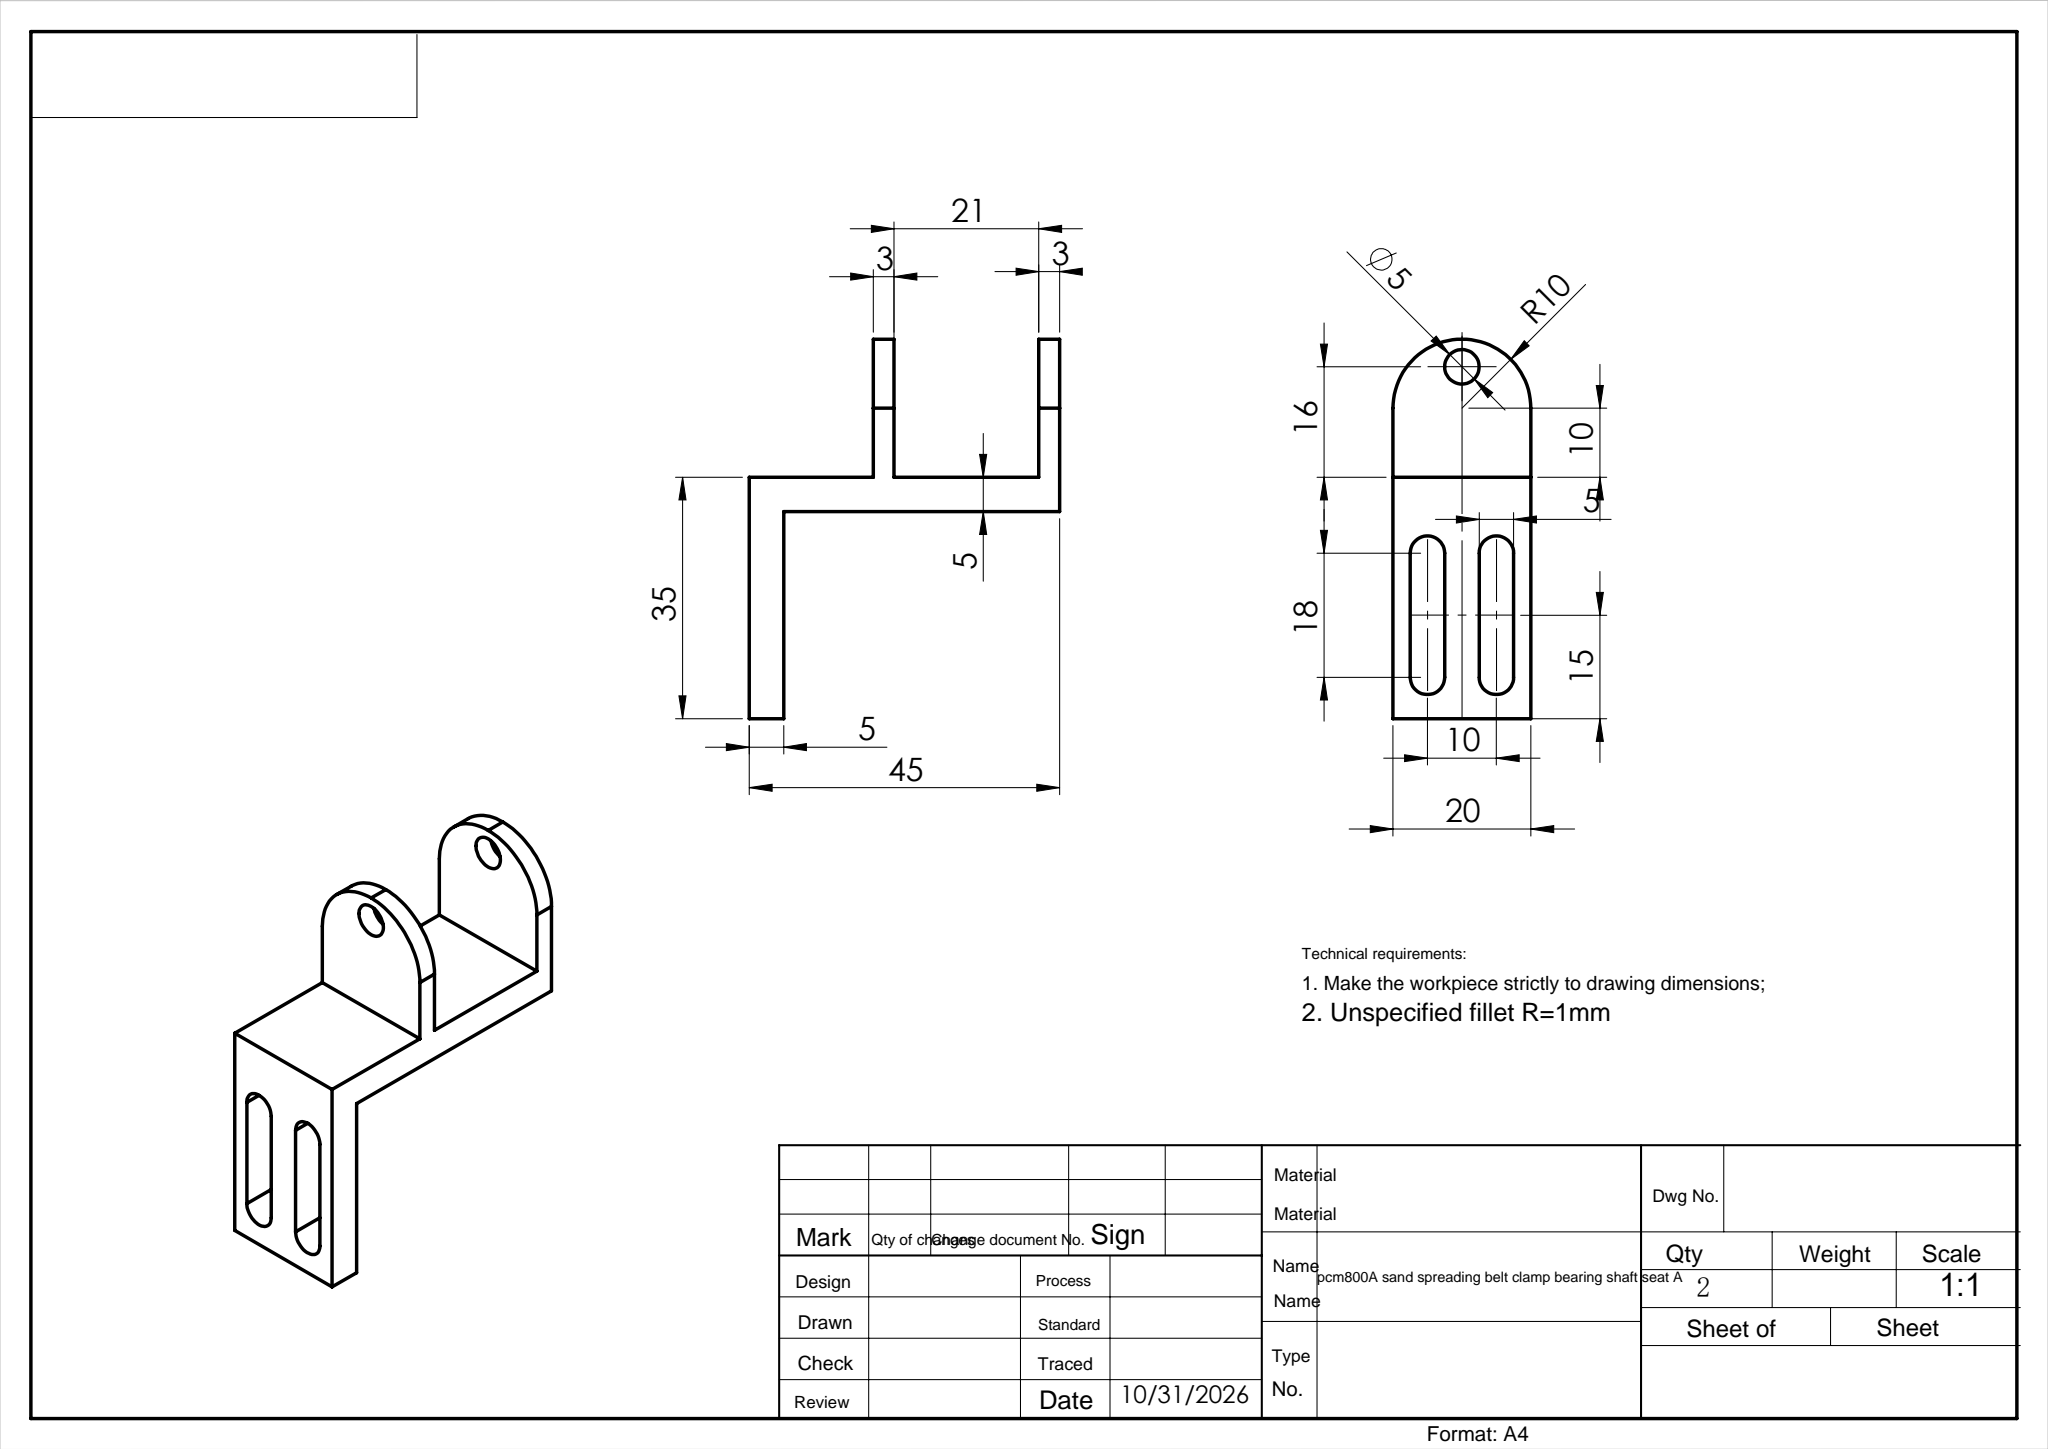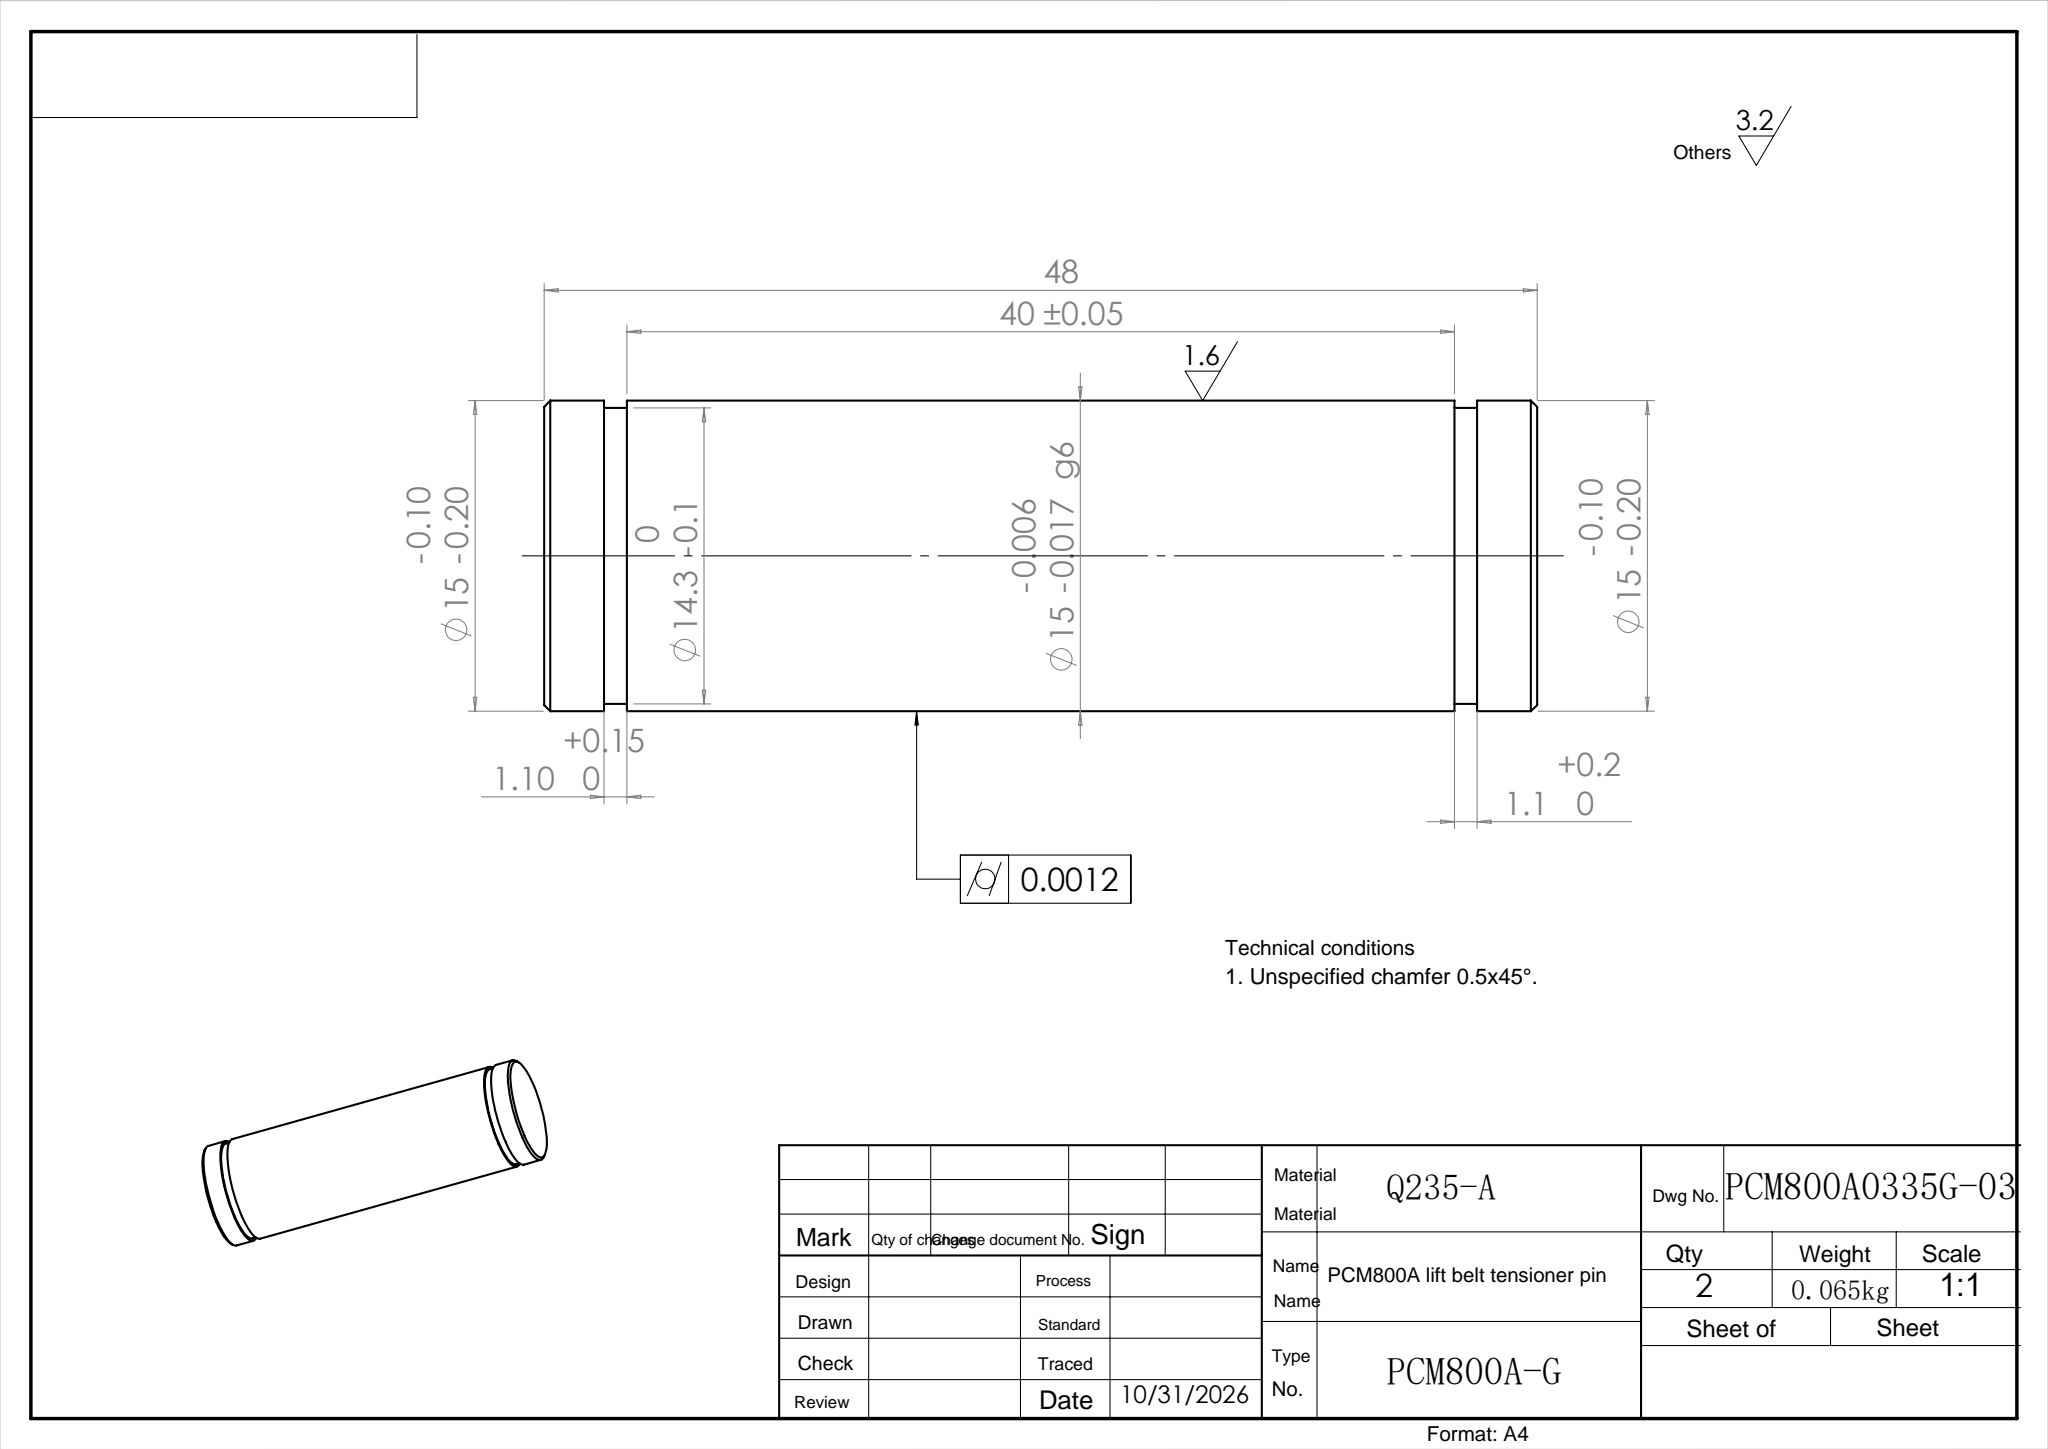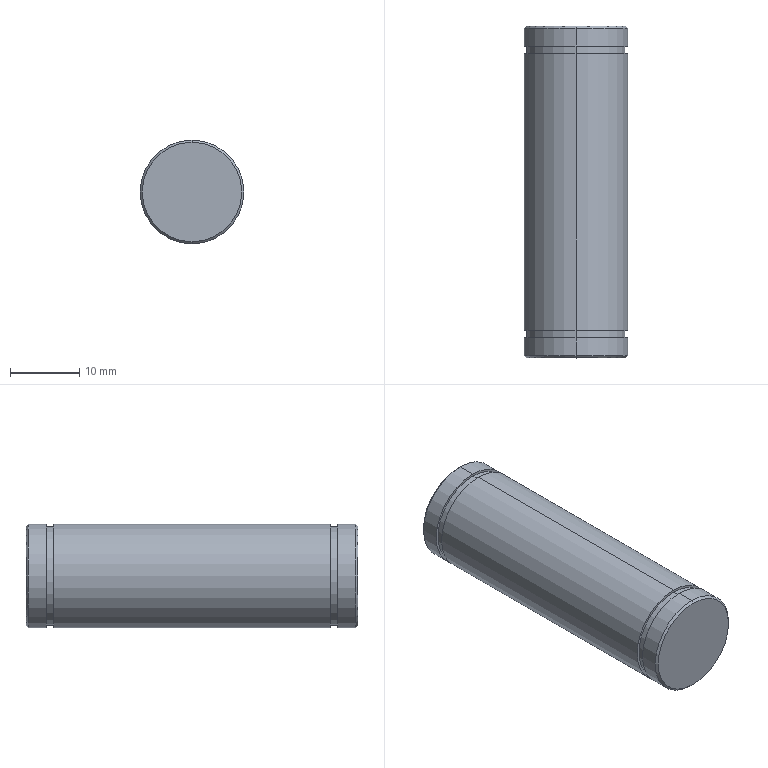Part | SolidWorks | features MirrorStock 1 | 1 solid | 20 faces | box 15 x 48 x 15 mm | volume 8443 mm3 | cylinder 10 | plane 6 | cone 4 | commonest cylinder face diameters 15 x6 14.3 x4
STEP:
#1=CARTESIAN_POINT('',(0.,48.,7.2));
#2=VERTEX_POINT('',#1);
#3=CARTESIAN_POINT('',(0.,48.,-7.2));
#4=VERTEX_POINT('',#3);
#5=CARTESIAN_POINT('',(0.,48.,0.));
#6=DIRECTION('',(0.,-1.,0.));
#7=DIRECTION('',(0.,0.,-1.));
#8=AXIS2_PLACEMENT_3D('',#5,#6,#7);
#9=CIRCLE('',#8,7.2);
#10=EDGE_CURVE('',#2,#4,#9,.T.);
#11=ORIENTED_EDGE('',*,*,#10,.T.);
#12=CARTESIAN_POINT('',(0.,47.7,-7.5));
#13=VERTEX_POINT('',#12);
#14=CARTESIAN_POINT('',(0.,48.,-7.2));
#15=DIRECTION('',(0.,-0.7071,-0.7071));
#16=VECTOR('',#15,1000.);
#17=LINE('',#14,#16);
#18=EDGE_CURVE('',#4,#13,#17,.T.);
#19=ORIENTED_EDGE('',*,*,#18,.T.);
#20=CARTESIAN_POINT('',(0.,47.7,7.5));
#21=VERTEX_POINT('',#20);
#22=CARTESIAN_POINT('',(0.,47.7,0.));
#23=DIRECTION('',(0.,1.,0.));
#24=DIRECTION('',(0.,0.,-1.));
#25=AXIS2_PLACEMENT_3D('',#22,#23,#24);
#26=CIRCLE('',#25,7.5);
#27=EDGE_CURVE('',#13,#21,#26,.T.);
#28=ORIENTED_EDGE('',*,*,#27,.T.);
#29=CARTESIAN_POINT('',(0.,48.,7.2));
#30=DIRECTION('',(0.,-0.7071,0.7071));
#31=VECTOR('',#30,1000.);
#32=LINE('',#29,#31);
#33=EDGE_CURVE('',#2,#21,#32,.T.);
#34=ORIENTED_EDGE('',*,*,#33,.F.);
#35=EDGE_LOOP('',(#11,#19,#28,#34));
#36=FACE_OUTER_BOUND('',#35,.T.);
#37=CARTESIAN_POINT('',(0.,48.,0.));
#38=DIRECTION('',(0.,-1.,0.));
#39=DIRECTION('',(0.,0.,1.));
#40=AXIS2_PLACEMENT_3D('',#37,#38,#39);
#41=CONICAL_SURFACE('',#40,7.2,0.7854);
#42=ADVANCED_FACE('',(#36),#41,.T.);
#43=CARTESIAN_POINT('',(0.,0.,-7.2));
#44=VERTEX_POINT('',#43);
#45=CARTESIAN_POINT('',(0.,0.,7.2));
#46=VERTEX_POINT('',#45);
#47=CARTESIAN_POINT('',(0.,0.,0.));
#48=DIRECTION('',(0.,1.,0.));
#49=DIRECTION('',(0.,0.,-1.));
#50=AXIS2_PLACEMENT_3D('',#47,#48,#49);
#51=CIRCLE('',#50,7.2);
#52=EDGE_CURVE('',#44,#46,#51,.T.);
#53=ORIENTED_EDGE('',*,*,#52,.T.);
#54=CARTESIAN_POINT('',(0.,0.3,7.5));
#55=VERTEX_POINT('',#54);
#56=CARTESIAN_POINT('',(0.,0.3,7.5));
#57=DIRECTION('',(0.,0.7071,0.7071));
#58=VECTOR('',#57,1000.);
#59=LINE('',#56,#58);
#60=EDGE_CURVE('',#46,#55,#59,.T.);
#61=ORIENTED_EDGE('',*,*,#60,.T.);
#62=CARTESIAN_POINT('',(0.,0.3,-7.5));
#63=VERTEX_POINT('',#62);
#64=CARTESIAN_POINT('',(0.,0.3,0.));
#65=DIRECTION('',(0.,-1.,0.));
#66=DIRECTION('',(0.,0.,-1.));
#67=AXIS2_PLACEMENT_3D('',#64,#65,#66);
#68=CIRCLE('',#67,7.5);
#69=EDGE_CURVE('',#55,#63,#68,.T.);
#70=ORIENTED_EDGE('',*,*,#69,.T.);
#71=CARTESIAN_POINT('',(0.,0.3,-7.5));
#72=DIRECTION('',(0.,0.7071,-0.7071));
#73=VECTOR('',#72,1000.);
#74=LINE('',#71,#73);
#75=EDGE_CURVE('',#44,#63,#74,.T.);
#76=ORIENTED_EDGE('',*,*,#75,.F.);
#77=EDGE_LOOP('',(#53,#61,#70,#76));
#78=FACE_OUTER_BOUND('',#77,.T.);
#79=CARTESIAN_POINT('',(0.,0.3,0.));
#80=DIRECTION('',(0.,1.,0.));
#81=DIRECTION('',(0.,0.,-1.));
#82=AXIS2_PLACEMENT_3D('',#79,#80,#81);
#83=CONICAL_SURFACE('',#82,7.5,0.7854);
#84=ADVANCED_FACE('',(#78),#83,.T.);
#85=ORIENTED_EDGE('',*,*,#27,.F.);
#86=CARTESIAN_POINT('',(0.,45.1,-7.5));
#87=VERTEX_POINT('',#86);
#88=CARTESIAN_POINT('',(0.,48.,-7.5));
#89=DIRECTION('',(0.,-1.,0.));
#90=VECTOR('',#89,1000.);
#91=LINE('',#88,#90);
#92=EDGE_CURVE('',#13,#87,#91,.T.);
#93=ORIENTED_EDGE('',*,*,#92,.T.);
#94=CARTESIAN_POINT('',(0.,45.1,7.5));
#95=VERTEX_POINT('',#94);
#96=CARTESIAN_POINT('',(0.,45.1,0.));
#97=DIRECTION('',(0.,-1.,0.));
#98=DIRECTION('',(0.,0.,-1.));
#99=AXIS2_PLACEMENT_3D('',#96,#97,#98);
#100=CIRCLE('',#99,7.5);
#101=EDGE_CURVE('',#95,#87,#100,.T.);
#102=ORIENTED_EDGE('',*,*,#101,.F.);
#103=CARTESIAN_POINT('',(0.,48.,7.5));
#104=DIRECTION('',(0.,-1.,0.));
#105=VECTOR('',#104,1000.);
#106=LINE('',#103,#105);
#107=EDGE_CURVE('',#21,#95,#106,.T.);
#108=ORIENTED_EDGE('',*,*,#107,.F.);
#109=EDGE_LOOP('',(#85,#93,#102,#108));
#110=FACE_OUTER_BOUND('',#109,.T.);
#111=CARTESIAN_POINT('',(0.,48.,0.));
#112=DIRECTION('',(0.,-1.,0.));
#113=DIRECTION('',(0.,0.,1.));
#114=AXIS2_PLACEMENT_3D('',#111,#112,#113);
#115=CYLINDRICAL_SURFACE('',#114,7.5);
#116=ADVANCED_FACE('',(#110),#115,.T.);
#117=CARTESIAN_POINT('',(0.,45.1,7.15));
#118=VERTEX_POINT('',#117);
#119=CARTESIAN_POINT('',(0.,45.1,-7.15));
#120=VERTEX_POINT('',#119);
#121=CARTESIAN_POINT('',(0.,45.1,0.));
#122=DIRECTION('',(0.,-1.,0.));
#123=DIRECTION('',(0.,0.,-1.));
#124=AXIS2_PLACEMENT_3D('',#121,#122,#123);
#125=CIRCLE('',#124,7.15);
#126=EDGE_CURVE('',#118,#120,#125,.T.);
#127=ORIENTED_EDGE('',*,*,#126,.T.);
#128=CARTESIAN_POINT('',(0.,44.,-7.15));
#129=VERTEX_POINT('',#128);
#130=CARTESIAN_POINT('',(0.,45.1,-7.15));
#131=DIRECTION('',(0.,-1.,0.));
#132=VECTOR('',#131,1000.);
#133=LINE('',#130,#132);
#134=EDGE_CURVE('',#120,#129,#133,.T.);
#135=ORIENTED_EDGE('',*,*,#134,.T.);
#136=CARTESIAN_POINT('',(0.,44.,7.15));
#137=VERTEX_POINT('',#136);
#138=CARTESIAN_POINT('',(0.,44.,0.));
#139=DIRECTION('',(0.,-1.,0.));
#140=DIRECTION('',(0.,0.,-1.));
#141=AXIS2_PLACEMENT_3D('',#138,#139,#140);
#142=CIRCLE('',#141,7.15);
#143=EDGE_CURVE('',#137,#129,#142,.T.);
#144=ORIENTED_EDGE('',*,*,#143,.F.);
#145=CARTESIAN_POINT('',(0.,45.1,7.15));
#146=DIRECTION('',(0.,-1.,0.));
#147=VECTOR('',#146,1000.);
#148=LINE('',#145,#147);
#149=EDGE_CURVE('',#118,#137,#148,.T.);
#150=ORIENTED_EDGE('',*,*,#149,.F.);
#151=EDGE_LOOP('',(#127,#135,#144,#150));
#152=FACE_OUTER_BOUND('',#151,.T.);
#153=CARTESIAN_POINT('',(0.,45.1,0.));
#154=DIRECTION('',(0.,-1.,0.));
#155=DIRECTION('',(0.,0.,1.));
#156=AXIS2_PLACEMENT_3D('',#153,#154,#155);
#157=CYLINDRICAL_SURFACE('',#156,7.15);
#158=ADVANCED_FACE('',(#152),#157,.T.);
#159=CARTESIAN_POINT('',(0.,44.,7.5));
#160=VERTEX_POINT('',#159);
#161=CARTESIAN_POINT('',(0.,44.,-7.5));
#162=VERTEX_POINT('',#161);
#163=CARTESIAN_POINT('',(0.,44.,0.));
#164=DIRECTION('',(0.,-1.,0.));
#165=DIRECTION('',(0.,0.,-1.));
#166=AXIS2_PLACEMENT_3D('',#163,#164,#165);
#167=CIRCLE('',#166,7.5);
#168=EDGE_CURVE('',#160,#162,#167,.T.);
#169=ORIENTED_EDGE('',*,*,#168,.T.);
#170=CARTESIAN_POINT('',(0.,4.,-7.5));
#171=VERTEX_POINT('',#170);
#172=CARTESIAN_POINT('',(0.,44.,-7.5));
#173=DIRECTION('',(0.,-1.,0.));
#174=VECTOR('',#173,1000.);
#175=LINE('',#172,#174);
#176=EDGE_CURVE('',#162,#171,#175,.T.);
#177=ORIENTED_EDGE('',*,*,#176,.T.);
#178=CARTESIAN_POINT('',(0.,4.,7.5));
#179=VERTEX_POINT('',#178);
#180=CARTESIAN_POINT('',(0.,4.,0.));
#181=DIRECTION('',(0.,-1.,0.));
#182=DIRECTION('',(0.,0.,-1.));
#183=AXIS2_PLACEMENT_3D('',#180,#181,#182);
#184=CIRCLE('',#183,7.5);
#185=EDGE_CURVE('',#179,#171,#184,.T.);
#186=ORIENTED_EDGE('',*,*,#185,.F.);
#187=CARTESIAN_POINT('',(0.,44.,7.5));
#188=DIRECTION('',(0.,-1.,0.));
#189=VECTOR('',#188,1000.);
#190=LINE('',#187,#189);
#191=EDGE_CURVE('',#160,#179,#190,.T.);
#192=ORIENTED_EDGE('',*,*,#191,.F.);
#193=EDGE_LOOP('',(#169,#177,#186,#192));
#194=FACE_OUTER_BOUND('',#193,.T.);
#195=CARTESIAN_POINT('',(0.,44.,0.));
#196=DIRECTION('',(0.,-1.,0.));
#197=DIRECTION('',(0.,0.,1.));
#198=AXIS2_PLACEMENT_3D('',#195,#196,#197);
#199=CYLINDRICAL_SURFACE('',#198,7.5);
#200=ADVANCED_FACE('',(#194),#199,.T.);
#201=CARTESIAN_POINT('',(0.,4.,7.15));
#202=VERTEX_POINT('',#201);
#203=CARTESIAN_POINT('',(0.,4.,-7.15));
#204=VERTEX_POINT('',#203);
#205=CARTESIAN_POINT('',(0.,4.,0.));
#206=DIRECTION('',(0.,-1.,0.));
#207=DIRECTION('',(0.,0.,-1.));
#208=AXIS2_PLACEMENT_3D('',#205,#206,#207);
#209=CIRCLE('',#208,7.15);
#210=EDGE_CURVE('',#202,#204,#209,.T.);
#211=ORIENTED_EDGE('',*,*,#210,.T.);
#212=CARTESIAN_POINT('',(0.,2.9,-7.15));
#213=VERTEX_POINT('',#212);
#214=CARTESIAN_POINT('',(0.,4.,-7.15));
#215=DIRECTION('',(0.,-1.,0.));
#216=VECTOR('',#215,1000.);
#217=LINE('',#214,#216);
#218=EDGE_CURVE('',#204,#213,#217,.T.);
#219=ORIENTED_EDGE('',*,*,#218,.T.);
#220=CARTESIAN_POINT('',(0.,2.9,7.15));
#221=VERTEX_POINT('',#220);
#222=CARTESIAN_POINT('',(0.,2.9,0.));
#223=DIRECTION('',(0.,-1.,0.));
#224=DIRECTION('',(0.,0.,-1.));
#225=AXIS2_PLACEMENT_3D('',#222,#223,#224);
#226=CIRCLE('',#225,7.15);
#227=EDGE_CURVE('',#221,#213,#226,.T.);
#228=ORIENTED_EDGE('',*,*,#227,.F.);
#229=CARTESIAN_POINT('',(0.,4.,7.15));
#230=DIRECTION('',(0.,-1.,0.));
#231=VECTOR('',#230,1000.);
#232=LINE('',#229,#231);
#233=EDGE_CURVE('',#202,#221,#232,.T.);
#234=ORIENTED_EDGE('',*,*,#233,.F.);
#235=EDGE_LOOP('',(#211,#219,#228,#234));
#236=FACE_OUTER_BOUND('',#235,.T.);
#237=CARTESIAN_POINT('',(0.,4.,0.));
#238=DIRECTION('',(0.,-1.,0.));
#239=DIRECTION('',(0.,0.,1.));
#240=AXIS2_PLACEMENT_3D('',#237,#238,#239);
#241=CYLINDRICAL_SURFACE('',#240,7.15);
#242=ADVANCED_FACE('',(#236),#241,.T.);
#243=CARTESIAN_POINT('',(0.,2.9,7.5));
#244=VERTEX_POINT('',#243);
#245=CARTESIAN_POINT('',(0.,2.9,-7.5));
#246=VERTEX_POINT('',#245);
#247=CARTESIAN_POINT('',(0.,2.9,0.));
#248=DIRECTION('',(0.,-1.,0.));
#249=DIRECTION('',(0.,0.,-1.));
#250=AXIS2_PLACEMENT_3D('',#247,#248,#249);
#251=CIRCLE('',#250,7.5);
#252=EDGE_CURVE('',#244,#246,#251,.T.);
#253=ORIENTED_EDGE('',*,*,#252,.T.);
#254=CARTESIAN_POINT('',(0.,2.9,-7.5));
#255=DIRECTION('',(0.,-1.,0.));
#256=VECTOR('',#255,1000.);
#257=LINE('',#254,#256);
#258=EDGE_CURVE('',#246,#63,#257,.T.);
#259=ORIENTED_EDGE('',*,*,#258,.T.);
#260=ORIENTED_EDGE('',*,*,#69,.F.);
#261=CARTESIAN_POINT('',(0.,2.9,7.5));
#262=DIRECTION('',(0.,-1.,0.));
#263=VECTOR('',#262,1000.);
#264=LINE('',#261,#263);
#265=EDGE_CURVE('',#244,#55,#264,.T.);
#266=ORIENTED_EDGE('',*,*,#265,.F.);
#267=EDGE_LOOP('',(#253,#259,#260,#266));
#268=FACE_OUTER_BOUND('',#267,.T.);
#269=CARTESIAN_POINT('',(0.,2.9,0.));
#270=DIRECTION('',(0.,-1.,0.));
#271=DIRECTION('',(0.,0.,1.));
#272=AXIS2_PLACEMENT_3D('',#269,#270,#271);
#273=CYLINDRICAL_SURFACE('',#272,7.5);
#274=ADVANCED_FACE('',(#268),#273,.T.);
#275=ORIENTED_EDGE('',*,*,#168,.F.);
#276=CARTESIAN_POINT('',(0.,44.,0.));
#277=DIRECTION('',(0.,-1.,0.));
#278=DIRECTION('',(0.,0.,-1.));
#279=AXIS2_PLACEMENT_3D('',#276,#277,#278);
#280=CIRCLE('',#279,7.5);
#281=EDGE_CURVE('',#162,#160,#280,.T.);
#282=ORIENTED_EDGE('',*,*,#281,.F.);
#283=EDGE_LOOP('',(#275,#282));
#284=FACE_OUTER_BOUND('',#283,.T.);
#285=ORIENTED_EDGE('',*,*,#143,.T.);
#286=CARTESIAN_POINT('',(0.,44.,0.));
#287=DIRECTION('',(0.,-1.,0.));
#288=DIRECTION('',(0.,0.,-1.));
#289=AXIS2_PLACEMENT_3D('',#286,#287,#288);
#290=CIRCLE('',#289,7.15);
#291=EDGE_CURVE('',#129,#137,#290,.T.);
#292=ORIENTED_EDGE('',*,*,#291,.T.);
#293=EDGE_LOOP('',(#285,#292));
#294=FACE_BOUND('',#293,.T.);
#295=CARTESIAN_POINT('',(0.,44.,0.));
#296=DIRECTION('',(0.,1.,0.));
#297=DIRECTION('',(0.,0.,-1.));
#298=AXIS2_PLACEMENT_3D('',#295,#296,#297);
#299=PLANE('',#298);
#300=ADVANCED_FACE('',(#284,#294),#299,.T.);
#301=ORIENTED_EDGE('',*,*,#252,.F.);
#302=CARTESIAN_POINT('',(0.,2.9,0.));
#303=DIRECTION('',(0.,-1.,0.));
#304=DIRECTION('',(0.,0.,-1.));
#305=AXIS2_PLACEMENT_3D('',#302,#303,#304);
#306=CIRCLE('',#305,7.5);
#307=EDGE_CURVE('',#246,#244,#306,.T.);
#308=ORIENTED_EDGE('',*,*,#307,.F.);
#309=EDGE_LOOP('',(#301,#308));
#310=FACE_OUTER_BOUND('',#309,.T.);
#311=ORIENTED_EDGE('',*,*,#227,.T.);
#312=CARTESIAN_POINT('',(0.,2.9,0.));
#313=DIRECTION('',(0.,-1.,0.));
#314=DIRECTION('',(0.,0.,-1.));
#315=AXIS2_PLACEMENT_3D('',#312,#313,#314);
#316=CIRCLE('',#315,7.15);
#317=EDGE_CURVE('',#213,#221,#316,.T.);
#318=ORIENTED_EDGE('',*,*,#317,.T.);
#319=EDGE_LOOP('',(#311,#318));
#320=FACE_BOUND('',#319,.T.);
#321=CARTESIAN_POINT('',(0.,2.9,0.));
#322=DIRECTION('',(0.,1.,0.));
#323=DIRECTION('',(0.,0.,-1.));
#324=AXIS2_PLACEMENT_3D('',#321,#322,#323);
#325=PLANE('',#324);
#326=ADVANCED_FACE('',(#310,#320),#325,.T.);
#327=ORIENTED_EDGE('',*,*,#258,.F.);
#328=ORIENTED_EDGE('',*,*,#307,.T.);
#329=ORIENTED_EDGE('',*,*,#265,.T.);
#330=CARTESIAN_POINT('',(0.,0.3,0.));
#331=DIRECTION('',(0.,-1.,0.));
#332=DIRECTION('',(0.,0.,-1.));
#333=AXIS2_PLACEMENT_3D('',#330,#331,#332);
#334=CIRCLE('',#333,7.5);
#335=EDGE_CURVE('',#63,#55,#334,.T.);
#336=ORIENTED_EDGE('',*,*,#335,.F.);
#337=EDGE_LOOP('',(#327,#328,#329,#336));
#338=FACE_OUTER_BOUND('',#337,.T.);
#339=CARTESIAN_POINT('',(0.,2.9,0.));
#340=DIRECTION('',(0.,-1.,0.));
#341=DIRECTION('',(0.,0.,1.));
#342=AXIS2_PLACEMENT_3D('',#339,#340,#341);
#343=CYLINDRICAL_SURFACE('',#342,7.5);
#344=ADVANCED_FACE('',(#338),#343,.T.);
#345=ORIENTED_EDGE('',*,*,#52,.F.);
#346=CARTESIAN_POINT('',(0.,0.,0.));
#347=DIRECTION('',(0.,1.,0.));
#348=DIRECTION('',(0.,0.,-1.));
#349=AXIS2_PLACEMENT_3D('',#346,#347,#348);
#350=CIRCLE('',#349,7.2);
#351=EDGE_CURVE('',#46,#44,#350,.T.);
#352=ORIENTED_EDGE('',*,*,#351,.F.);
#353=EDGE_LOOP('',(#345,#352));
#354=FACE_OUTER_BOUND('',#353,.T.);
#355=CARTESIAN_POINT('',(0.,0.,0.));
#356=DIRECTION('',(0.,1.,0.));
#357=DIRECTION('',(0.,0.,-1.));
#358=AXIS2_PLACEMENT_3D('',#355,#356,#357);
#359=PLANE('',#358);
#360=ADVANCED_FACE('',(#354),#359,.F.);
#361=ORIENTED_EDGE('',*,*,#218,.F.);
#362=CARTESIAN_POINT('',(0.,4.,0.));
#363=DIRECTION('',(0.,-1.,0.));
#364=DIRECTION('',(0.,0.,-1.));
#365=AXIS2_PLACEMENT_3D('',#362,#363,#364);
#366=CIRCLE('',#365,7.15);
#367=EDGE_CURVE('',#204,#202,#366,.T.);
#368=ORIENTED_EDGE('',*,*,#367,.T.);
#369=ORIENTED_EDGE('',*,*,#233,.T.);
#370=ORIENTED_EDGE('',*,*,#317,.F.);
#371=EDGE_LOOP('',(#361,#368,#369,#370));
#372=FACE_OUTER_BOUND('',#371,.T.);
#373=CARTESIAN_POINT('',(0.,4.,0.));
#374=DIRECTION('',(0.,-1.,0.));
#375=DIRECTION('',(0.,0.,1.));
#376=AXIS2_PLACEMENT_3D('',#373,#374,#375);
#377=CYLINDRICAL_SURFACE('',#376,7.15);
#378=ADVANCED_FACE('',(#372),#377,.T.);
#379=ORIENTED_EDGE('',*,*,#185,.T.);
#380=CARTESIAN_POINT('',(0.,4.,0.));
#381=DIRECTION('',(0.,-1.,0.));
#382=DIRECTION('',(0.,0.,-1.));
#383=AXIS2_PLACEMENT_3D('',#380,#381,#382);
#384=CIRCLE('',#383,7.5);
#385=EDGE_CURVE('',#171,#179,#384,.T.);
#386=ORIENTED_EDGE('',*,*,#385,.T.);
#387=EDGE_LOOP('',(#379,#386));
#388=FACE_OUTER_BOUND('',#387,.T.);
#389=ORIENTED_EDGE('',*,*,#210,.F.);
#390=ORIENTED_EDGE('',*,*,#367,.F.);
#391=EDGE_LOOP('',(#389,#390));
#392=FACE_BOUND('',#391,.T.);
#393=CARTESIAN_POINT('',(0.,4.,0.));
#394=DIRECTION('',(0.,1.,0.));
#395=DIRECTION('',(0.,0.,-1.));
#396=AXIS2_PLACEMENT_3D('',#393,#394,#395);
#397=PLANE('',#396);
#398=ADVANCED_FACE('',(#388,#392),#397,.F.);
#399=ORIENTED_EDGE('',*,*,#176,.F.);
#400=ORIENTED_EDGE('',*,*,#281,.T.);
#401=ORIENTED_EDGE('',*,*,#191,.T.);
#402=ORIENTED_EDGE('',*,*,#385,.F.);
#403=EDGE_LOOP('',(#399,#400,#401,#402));
#404=FACE_OUTER_BOUND('',#403,.T.);
#405=CARTESIAN_POINT('',(0.,44.,0.));
#406=DIRECTION('',(0.,-1.,0.));
#407=DIRECTION('',(0.,0.,1.));
#408=AXIS2_PLACEMENT_3D('',#405,#406,#407);
#409=CYLINDRICAL_SURFACE('',#408,7.5);
#410=ADVANCED_FACE('',(#404),#409,.T.);
#411=ORIENTED_EDGE('',*,*,#134,.F.);
#412=CARTESIAN_POINT('',(0.,45.1,0.));
#413=DIRECTION('',(0.,-1.,0.));
#414=DIRECTION('',(0.,0.,-1.));
#415=AXIS2_PLACEMENT_3D('',#412,#413,#414);
#416=CIRCLE('',#415,7.15);
#417=EDGE_CURVE('',#120,#118,#416,.T.);
#418=ORIENTED_EDGE('',*,*,#417,.T.);
#419=ORIENTED_EDGE('',*,*,#149,.T.);
#420=ORIENTED_EDGE('',*,*,#291,.F.);
#421=EDGE_LOOP('',(#411,#418,#419,#420));
#422=FACE_OUTER_BOUND('',#421,.T.);
#423=CARTESIAN_POINT('',(0.,45.1,0.));
#424=DIRECTION('',(0.,-1.,0.));
#425=DIRECTION('',(0.,0.,1.));
#426=AXIS2_PLACEMENT_3D('',#423,#424,#425);
#427=CYLINDRICAL_SURFACE('',#426,7.15);
#428=ADVANCED_FACE('',(#422),#427,.T.);
#429=ORIENTED_EDGE('',*,*,#101,.T.);
#430=CARTESIAN_POINT('',(0.,45.1,0.));
#431=DIRECTION('',(0.,-1.,0.));
#432=DIRECTION('',(0.,0.,-1.));
#433=AXIS2_PLACEMENT_3D('',#430,#431,#432);
#434=CIRCLE('',#433,7.5);
#435=EDGE_CURVE('',#87,#95,#434,.T.);
#436=ORIENTED_EDGE('',*,*,#435,.T.);
#437=EDGE_LOOP('',(#429,#436));
#438=FACE_OUTER_BOUND('',#437,.T.);
#439=ORIENTED_EDGE('',*,*,#126,.F.);
#440=ORIENTED_EDGE('',*,*,#417,.F.);
#441=EDGE_LOOP('',(#439,#440));
#442=FACE_BOUND('',#441,.T.);
#443=CARTESIAN_POINT('',(0.,45.1,0.));
#444=DIRECTION('',(0.,1.,0.));
#445=DIRECTION('',(0.,0.,-1.));
#446=AXIS2_PLACEMENT_3D('',#443,#444,#445);
#447=PLANE('',#446);
#448=ADVANCED_FACE('',(#438,#442),#447,.F.);
#449=ORIENTED_EDGE('',*,*,#92,.F.);
#450=CARTESIAN_POINT('',(0.,47.7,0.));
#451=DIRECTION('',(0.,1.,0.));
#452=DIRECTION('',(0.,0.,-1.));
#453=AXIS2_PLACEMENT_3D('',#450,#451,#452);
#454=CIRCLE('',#453,7.5);
#455=EDGE_CURVE('',#21,#13,#454,.T.);
#456=ORIENTED_EDGE('',*,*,#455,.F.);
#457=ORIENTED_EDGE('',*,*,#107,.T.);
#458=ORIENTED_EDGE('',*,*,#435,.F.);
#459=EDGE_LOOP('',(#449,#456,#457,#458));
#460=FACE_OUTER_BOUND('',#459,.T.);
#461=CARTESIAN_POINT('',(0.,48.,0.));
#462=DIRECTION('',(0.,-1.,0.));
#463=DIRECTION('',(0.,0.,1.));
#464=AXIS2_PLACEMENT_3D('',#461,#462,#463);
#465=CYLINDRICAL_SURFACE('',#464,7.5);
#466=ADVANCED_FACE('',(#460),#465,.T.);
#467=ORIENTED_EDGE('',*,*,#10,.F.);
#468=CARTESIAN_POINT('',(0.,48.,0.));
#469=DIRECTION('',(0.,-1.,0.));
#470=DIRECTION('',(0.,0.,-1.));
#471=AXIS2_PLACEMENT_3D('',#468,#469,#470);
#472=CIRCLE('',#471,7.2);
#473=EDGE_CURVE('',#4,#2,#472,.T.);
#474=ORIENTED_EDGE('',*,*,#473,.F.);
#475=EDGE_LOOP('',(#467,#474));
#476=FACE_OUTER_BOUND('',#475,.T.);
#477=CARTESIAN_POINT('',(0.,48.,0.));
#478=DIRECTION('',(0.,1.,0.));
#479=DIRECTION('',(0.,0.,-1.));
#480=AXIS2_PLACEMENT_3D('',#477,#478,#479);
#481=PLANE('',#480);
#482=ADVANCED_FACE('',(#476),#481,.T.);
#483=ORIENTED_EDGE('',*,*,#60,.F.);
#484=ORIENTED_EDGE('',*,*,#351,.T.);
#485=ORIENTED_EDGE('',*,*,#75,.T.);
#486=ORIENTED_EDGE('',*,*,#335,.T.);
#487=EDGE_LOOP('',(#483,#484,#485,#486));
#488=FACE_OUTER_BOUND('',#487,.T.);
#489=CARTESIAN_POINT('',(0.,0.3,0.));
#490=DIRECTION('',(0.,1.,0.));
#491=DIRECTION('',(0.,0.,-1.));
#492=AXIS2_PLACEMENT_3D('',#489,#490,#491);
#493=CONICAL_SURFACE('',#492,7.5,0.7854);
#494=ADVANCED_FACE('',(#488),#493,.T.);
#495=ORIENTED_EDGE('',*,*,#18,.F.);
#496=ORIENTED_EDGE('',*,*,#473,.T.);
#497=ORIENTED_EDGE('',*,*,#33,.T.);
#498=ORIENTED_EDGE('',*,*,#455,.T.);
#499=EDGE_LOOP('',(#495,#496,#497,#498));
#500=FACE_OUTER_BOUND('',#499,.T.);
#501=CARTESIAN_POINT('',(0.,48.,0.));
#502=DIRECTION('',(0.,-1.,0.));
#503=DIRECTION('',(0.,0.,1.));
#504=AXIS2_PLACEMENT_3D('',#501,#502,#503);
#505=CONICAL_SURFACE('',#504,7.2,0.7854);
#506=ADVANCED_FACE('',(#500),#505,.T.);
#507=CLOSED_SHELL('',(#42,#84,#116,#158,#200,#242,#274,#300,#326,#344,#360,#378,#398,#410,#428,#448,#466,#482,#494,#506));
#508=MANIFOLD_SOLID_BREP('',#507);
#509=CARTESIAN_POINT('',(0.,0.,0.));
#510=DIRECTION('',(0.,0.,1.));
#511=DIRECTION('',(1.,0.,0.));
#512=AXIS2_PLACEMENT_3D('',#509,#510,#511);
#513=(LENGTH_UNIT()NAMED_UNIT(*)SI_UNIT(.MILLI.,.METRE.));
#514=UNCERTAINTY_MEASURE_WITH_UNIT(LENGTH_MEASURE(0.00001),#513,'','');
#515=(NAMED_UNIT(*)PLANE_ANGLE_UNIT()SI_UNIT($,.RADIAN.));
#516=(NAMED_UNIT(*)SI_UNIT($,.STERADIAN.)SOLID_ANGLE_UNIT());
#517=(GEOMETRIC_REPRESENTATION_CONTEXT(3)GLOBAL_UNCERTAINTY_ASSIGNED_CONTEXT((#514))GLOBAL_UNIT_ASSIGNED_CONTEXT((#513,#515,#516))REPRESENTATION_CONTEXT('',''));
#518=ADVANCED_BREP_SHAPE_REPRESENTATION('',(#508,#512),#517);